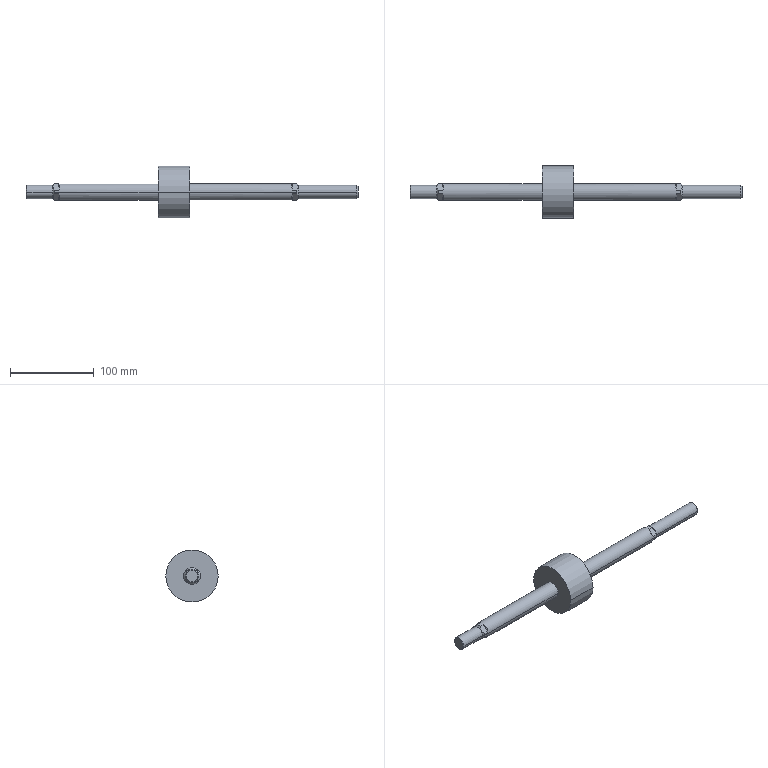Part | SolidWorks | features BaseBody 1 | 1 solid | 38 faces | box 397 x 62.5 x 62.5 mm | volume 216895 mm3 | plane 20 | cylinder 10 | cone 8 | commonest cylinder face diameters 16 x4 20 x4 62.5 x2
STEP:
#1=CARTESIAN_POINT('',(338.773,-8.,0.));
#2=VERTEX_POINT('',#1);
#3=CARTESIAN_POINT('',(338.773,8.,0.));
#4=VERTEX_POINT('',#3);
#5=CARTESIAN_POINT('',(338.773,0.,0.));
#6=DIRECTION('',(-1.,0.,0.));
#7=DIRECTION('',(0.,-1.,0.));
#8=AXIS2_PLACEMENT_3D('',#5,#6,#7);
#9=CIRCLE('',#8,8.);
#10=EDGE_CURVE('',#2,#4,#9,.T.);
#11=ORIENTED_EDGE('',*,*,#10,.T.);
#12=CARTESIAN_POINT('',(269.,8.,0.));
#13=VERTEX_POINT('',#12);
#14=CARTESIAN_POINT('',(340.,8.,0.));
#15=DIRECTION('',(-1.,0.,0.));
#16=VECTOR('',#15,1000.);
#17=LINE('',#14,#16);
#18=EDGE_CURVE('',#4,#13,#17,.T.);
#19=ORIENTED_EDGE('',*,*,#18,.T.);
#20=CARTESIAN_POINT('',(269.,-8.,0.));
#21=VERTEX_POINT('',#20);
#22=CARTESIAN_POINT('',(269.,0.,0.));
#23=DIRECTION('',(-1.,0.,0.));
#24=DIRECTION('',(0.,-1.,0.));
#25=AXIS2_PLACEMENT_3D('',#22,#23,#24);
#26=CIRCLE('',#25,8.);
#27=EDGE_CURVE('',#21,#13,#26,.T.);
#28=ORIENTED_EDGE('',*,*,#27,.F.);
#29=CARTESIAN_POINT('',(340.,-8.,0.));
#30=DIRECTION('',(-1.,0.,0.));
#31=VECTOR('',#30,1000.);
#32=LINE('',#29,#31);
#33=EDGE_CURVE('',#2,#21,#32,.T.);
#34=ORIENTED_EDGE('',*,*,#33,.F.);
#35=EDGE_LOOP('',(#11,#19,#28,#34));
#36=FACE_OUTER_BOUND('',#35,.T.);
#37=CARTESIAN_POINT('',(340.,0.,0.));
#38=DIRECTION('',(-1.,0.,0.));
#39=DIRECTION('',(0.,-1.,0.));
#40=AXIS2_PLACEMENT_3D('',#37,#38,#39);
#41=CYLINDRICAL_SURFACE('',#40,8.);
#42=ADVANCED_FACE('',(#36),#41,.T.);
#43=CARTESIAN_POINT('',(340.,-6.773,0.));
#44=VERTEX_POINT('',#43);
#45=CARTESIAN_POINT('',(340.,6.773,0.));
#46=VERTEX_POINT('',#45);
#47=CARTESIAN_POINT('',(340.,0.,0.));
#48=DIRECTION('',(-1.,0.,0.));
#49=DIRECTION('',(0.,-1.,0.));
#50=AXIS2_PLACEMENT_3D('',#47,#48,#49);
#51=CIRCLE('',#50,6.773);
#52=EDGE_CURVE('',#44,#46,#51,.T.);
#53=ORIENTED_EDGE('',*,*,#52,.T.);
#54=CARTESIAN_POINT('',(340.,6.773,0.));
#55=DIRECTION('',(-0.7071,0.7071,0.));
#56=VECTOR('',#55,1000.);
#57=LINE('',#54,#56);
#58=EDGE_CURVE('',#46,#4,#57,.T.);
#59=ORIENTED_EDGE('',*,*,#58,.T.);
#60=ORIENTED_EDGE('',*,*,#10,.F.);
#61=CARTESIAN_POINT('',(340.,-6.773,0.));
#62=DIRECTION('',(-0.7071,-0.7071,0.));
#63=VECTOR('',#62,1000.);
#64=LINE('',#61,#63);
#65=EDGE_CURVE('',#44,#2,#64,.T.);
#66=ORIENTED_EDGE('',*,*,#65,.F.);
#67=EDGE_LOOP('',(#53,#59,#60,#66));
#68=FACE_OUTER_BOUND('',#67,.T.);
#69=CARTESIAN_POINT('',(340.,0.,0.));
#70=DIRECTION('',(-1.,0.,0.));
#71=DIRECTION('',(0.,-1.,0.));
#72=AXIS2_PLACEMENT_3D('',#69,#70,#71);
#73=CONICAL_SURFACE('',#72,6.773,0.7854);
#74=ADVANCED_FACE('',(#68),#73,.T.);
#75=CARTESIAN_POINT('',(267.,9.735,2.285));
#76=VERTEX_POINT('',#75);
#77=CARTESIAN_POINT('',(267.,10.,0.));
#78=VERTEX_POINT('',#77);
#79=CARTESIAN_POINT('',(267.,0.,0.));
#80=DIRECTION('',(-1.,0.,0.));
#81=DIRECTION('',(0.,-1.,0.));
#82=AXIS2_PLACEMENT_3D('',#79,#80,#81);
#83=CIRCLE('',#82,10.);
#84=EDGE_CURVE('',#76,#78,#83,.T.);
#85=ORIENTED_EDGE('',*,*,#84,.T.);
#86=CARTESIAN_POINT('',(139.,10.,0.));
#87=VERTEX_POINT('',#86);
#88=CARTESIAN_POINT('',(340.,10.,0.));
#89=DIRECTION('',(-1.,0.,0.));
#90=VECTOR('',#89,1000.);
#91=LINE('',#88,#90);
#92=EDGE_CURVE('',#78,#87,#91,.T.);
#93=ORIENTED_EDGE('',*,*,#92,.T.);
#94=CARTESIAN_POINT('',(139.,-10.,0.));
#95=VERTEX_POINT('',#94);
#96=CARTESIAN_POINT('',(139.,0.,0.));
#97=DIRECTION('',(1.,0.,0.));
#98=DIRECTION('',(0.,-1.,0.));
#99=AXIS2_PLACEMENT_3D('',#96,#97,#98);
#100=CIRCLE('',#99,10.);
#101=EDGE_CURVE('',#87,#95,#100,.T.);
#102=ORIENTED_EDGE('',*,*,#101,.T.);
#103=CARTESIAN_POINT('',(267.,-10.,0.));
#104=VERTEX_POINT('',#103);
#105=CARTESIAN_POINT('',(340.,-10.,0.));
#106=DIRECTION('',(-1.,0.,0.));
#107=VECTOR('',#106,1000.);
#108=LINE('',#105,#107);
#109=EDGE_CURVE('',#104,#95,#108,.T.);
#110=ORIENTED_EDGE('',*,*,#109,.F.);
#111=CARTESIAN_POINT('',(267.,-9.735,2.285));
#112=VERTEX_POINT('',#111);
#113=CARTESIAN_POINT('',(267.,0.,0.));
#114=DIRECTION('',(-1.,0.,0.));
#115=DIRECTION('',(0.,-1.,0.));
#116=AXIS2_PLACEMENT_3D('',#113,#114,#115);
#117=CIRCLE('',#116,10.);
#118=EDGE_CURVE('',#104,#112,#117,.T.);
#119=ORIENTED_EDGE('',*,*,#118,.T.);
#120=CARTESIAN_POINT('',(262.,-9.735,2.285));
#121=VERTEX_POINT('',#120);
#122=CARTESIAN_POINT('',(340.,-9.735,2.285));
#123=DIRECTION('',(-1.,0.,0.));
#124=VECTOR('',#123,1000.);
#125=LINE('',#122,#124);
#126=EDGE_CURVE('',#112,#121,#125,.T.);
#127=ORIENTED_EDGE('',*,*,#126,.T.);
#128=CARTESIAN_POINT('',(262.,-2.285,9.735));
#129=VERTEX_POINT('',#128);
#130=CARTESIAN_POINT('',(262.,-9.735,2.285));
#131=CARTESIAN_POINT('',(259.944,-8.844,6.084));
#132=CARTESIAN_POINT('',(259.944,-6.084,8.844));
#133=CARTESIAN_POINT('',(262.,-2.285,9.735));
#134=(BOUNDED_CURVE()B_SPLINE_CURVE(3,(#130,#131,#132,#133),.UNSPECIFIED.,.F.,.F.)B_SPLINE_CURVE_WITH_KNOTS((4,4),(5.728,6.838),.UNSPECIFIED.)CURVE()GEOMETRIC_REPRESENTATION_ITEM()RATIONAL_B_SPLINE_CURVE((1.,0.9,0.9,1.))REPRESENTATION_ITEM(''));
#135=EDGE_CURVE('',#121,#129,#134,.T.);
#136=ORIENTED_EDGE('',*,*,#135,.T.);
#137=CARTESIAN_POINT('',(267.,-2.285,9.735));
#138=VERTEX_POINT('',#137);
#139=CARTESIAN_POINT('',(340.,-2.285,9.735));
#140=DIRECTION('',(1.,0.,0.));
#141=VECTOR('',#140,1000.);
#142=LINE('',#139,#141);
#143=EDGE_CURVE('',#129,#138,#142,.T.);
#144=ORIENTED_EDGE('',*,*,#143,.T.);
#145=CARTESIAN_POINT('',(267.,2.285,9.735));
#146=VERTEX_POINT('',#145);
#147=CARTESIAN_POINT('',(267.,0.,0.));
#148=DIRECTION('',(-1.,0.,0.));
#149=DIRECTION('',(0.,-1.,0.));
#150=AXIS2_PLACEMENT_3D('',#147,#148,#149);
#151=CIRCLE('',#150,10.);
#152=EDGE_CURVE('',#138,#146,#151,.T.);
#153=ORIENTED_EDGE('',*,*,#152,.T.);
#154=CARTESIAN_POINT('',(262.,2.285,9.735));
#155=VERTEX_POINT('',#154);
#156=CARTESIAN_POINT('',(340.,2.285,9.735));
#157=DIRECTION('',(-1.,0.,0.));
#158=VECTOR('',#157,1000.);
#159=LINE('',#156,#158);
#160=EDGE_CURVE('',#146,#155,#159,.T.);
#161=ORIENTED_EDGE('',*,*,#160,.T.);
#162=CARTESIAN_POINT('',(262.,9.735,2.285));
#163=VERTEX_POINT('',#162);
#164=CARTESIAN_POINT('',(262.,2.285,9.735));
#165=CARTESIAN_POINT('',(259.944,6.084,8.844));
#166=CARTESIAN_POINT('',(259.944,8.844,6.084));
#167=CARTESIAN_POINT('',(262.,9.735,2.285));
#168=(BOUNDED_CURVE()B_SPLINE_CURVE(3,(#164,#165,#166,#167),.UNSPECIFIED.,.F.,.F.)B_SPLINE_CURVE_WITH_KNOTS((4,4),(5.728,6.838),.UNSPECIFIED.)CURVE()GEOMETRIC_REPRESENTATION_ITEM()RATIONAL_B_SPLINE_CURVE((1.,0.9,0.9,1.))REPRESENTATION_ITEM(''));
#169=EDGE_CURVE('',#155,#163,#168,.T.);
#170=ORIENTED_EDGE('',*,*,#169,.T.);
#171=CARTESIAN_POINT('',(340.,9.735,2.285));
#172=DIRECTION('',(1.,0.,0.));
#173=VECTOR('',#172,1000.);
#174=LINE('',#171,#173);
#175=EDGE_CURVE('',#163,#76,#174,.T.);
#176=ORIENTED_EDGE('',*,*,#175,.T.);
#177=EDGE_LOOP('',(#85,#93,#102,#110,#119,#127,#136,#144,#153,#161,#170,#176));
#178=FACE_OUTER_BOUND('',#177,.T.);
#179=CARTESIAN_POINT('',(340.,0.,0.));
#180=DIRECTION('',(-1.,0.,0.));
#181=DIRECTION('',(0.,-1.,0.));
#182=AXIS2_PLACEMENT_3D('',#179,#180,#181);
#183=CYLINDRICAL_SURFACE('',#182,10.);
#184=ADVANCED_FACE('',(#178),#183,.T.);
#185=ORIENTED_EDGE('',*,*,#27,.T.);
#186=CARTESIAN_POINT('',(269.,8.,0.));
#187=DIRECTION('',(-0.7071,0.7071,0.));
#188=VECTOR('',#187,1000.);
#189=LINE('',#186,#188);
#190=EDGE_CURVE('',#13,#78,#189,.T.);
#191=ORIENTED_EDGE('',*,*,#190,.T.);
#192=ORIENTED_EDGE('',*,*,#84,.F.);
#193=CARTESIAN_POINT('',(267.,9.735,2.285));
#194=CARTESIAN_POINT('',(267.432,9.156,2.865));
#195=CARTESIAN_POINT('',(267.804,8.561,3.46));
#196=CARTESIAN_POINT('',(268.207,7.629,4.392));
#197=CARTESIAN_POINT('',(268.315,7.31,4.711));
#198=CARTESIAN_POINT('',(268.462,6.66,5.361));
#199=CARTESIAN_POINT('',(268.5,6.336,5.685));
#200=CARTESIAN_POINT('',(268.5,5.686,6.335));
#201=CARTESIAN_POINT('',(268.463,5.362,6.659));
#202=CARTESIAN_POINT('',(268.316,4.713,7.308));
#203=CARTESIAN_POINT('',(268.208,4.393,7.628));
#204=CARTESIAN_POINT('',(267.805,3.46,8.561));
#205=CARTESIAN_POINT('',(267.432,2.865,9.156));
#206=CARTESIAN_POINT('',(267.,2.285,9.735));
#207=B_SPLINE_CURVE_WITH_KNOTS('',3,(#193,#194,#195,#196,#197,#198,#199,#200,#201,#202,#203,#204,#205,#206),.UNSPECIFIED.,.F.,.F.,(4,2,2,2,2,2,4),(0.,0.002753,0.00413,0.005507,0.006884,0.00826,0.01101),.UNSPECIFIED.);
#208=EDGE_CURVE('',#76,#146,#207,.T.);
#209=ORIENTED_EDGE('',*,*,#208,.T.);
#210=ORIENTED_EDGE('',*,*,#152,.F.);
#211=CARTESIAN_POINT('',(267.,-2.285,9.735));
#212=CARTESIAN_POINT('',(267.432,-2.865,9.156));
#213=CARTESIAN_POINT('',(267.804,-3.46,8.561));
#214=CARTESIAN_POINT('',(268.207,-4.392,7.629));
#215=CARTESIAN_POINT('',(268.315,-4.711,7.31));
#216=CARTESIAN_POINT('',(268.462,-5.361,6.66));
#217=CARTESIAN_POINT('',(268.5,-5.685,6.336));
#218=CARTESIAN_POINT('',(268.5,-6.335,5.686));
#219=CARTESIAN_POINT('',(268.463,-6.659,5.362));
#220=CARTESIAN_POINT('',(268.316,-7.308,4.713));
#221=CARTESIAN_POINT('',(268.208,-7.628,4.393));
#222=CARTESIAN_POINT('',(267.805,-8.561,3.46));
#223=CARTESIAN_POINT('',(267.432,-9.156,2.865));
#224=CARTESIAN_POINT('',(267.,-9.735,2.285));
#225=B_SPLINE_CURVE_WITH_KNOTS('',3,(#211,#212,#213,#214,#215,#216,#217,#218,#219,#220,#221,#222,#223,#224),.UNSPECIFIED.,.F.,.F.,(4,2,2,2,2,2,4),(0.,0.002753,0.00413,0.005507,0.006884,0.00826,0.01101),.UNSPECIFIED.);
#226=EDGE_CURVE('',#138,#112,#225,.T.);
#227=ORIENTED_EDGE('',*,*,#226,.T.);
#228=ORIENTED_EDGE('',*,*,#118,.F.);
#229=CARTESIAN_POINT('',(269.,-8.,0.));
#230=DIRECTION('',(-0.7071,-0.7071,0.));
#231=VECTOR('',#230,1000.);
#232=LINE('',#229,#231);
#233=EDGE_CURVE('',#21,#104,#232,.T.);
#234=ORIENTED_EDGE('',*,*,#233,.F.);
#235=EDGE_LOOP('',(#185,#191,#192,#209,#210,#227,#228,#234));
#236=FACE_OUTER_BOUND('',#235,.T.);
#237=CARTESIAN_POINT('',(269.,0.,0.));
#238=DIRECTION('',(-1.,0.,0.));
#239=DIRECTION('',(0.,-1.,0.));
#240=AXIS2_PLACEMENT_3D('',#237,#238,#239);
#241=CONICAL_SURFACE('',#240,8.,0.7854);
#242=ADVANCED_FACE('',(#236),#241,.T.);
#243=CARTESIAN_POINT('',(139.,-31.25,0.));
#244=VERTEX_POINT('',#243);
#245=CARTESIAN_POINT('',(139.,31.25,0.));
#246=VERTEX_POINT('',#245);
#247=CARTESIAN_POINT('',(139.,0.,0.));
#248=DIRECTION('',(-1.,0.,0.));
#249=DIRECTION('',(0.,-1.,0.));
#250=AXIS2_PLACEMENT_3D('',#247,#248,#249);
#251=CIRCLE('',#250,31.25);
#252=EDGE_CURVE('',#244,#246,#251,.T.);
#253=ORIENTED_EDGE('',*,*,#252,.T.);
#254=CARTESIAN_POINT('',(101.,31.25,0.));
#255=VERTEX_POINT('',#254);
#256=CARTESIAN_POINT('',(139.,31.25,0.));
#257=DIRECTION('',(-1.,0.,0.));
#258=VECTOR('',#257,1000.);
#259=LINE('',#256,#258);
#260=EDGE_CURVE('',#246,#255,#259,.T.);
#261=ORIENTED_EDGE('',*,*,#260,.T.);
#262=CARTESIAN_POINT('',(101.,-31.25,0.));
#263=VERTEX_POINT('',#262);
#264=CARTESIAN_POINT('',(101.,0.,0.));
#265=DIRECTION('',(-1.,0.,0.));
#266=DIRECTION('',(0.,-1.,0.));
#267=AXIS2_PLACEMENT_3D('',#264,#265,#266);
#268=CIRCLE('',#267,31.25);
#269=EDGE_CURVE('',#263,#255,#268,.T.);
#270=ORIENTED_EDGE('',*,*,#269,.F.);
#271=CARTESIAN_POINT('',(139.,-31.25,0.));
#272=DIRECTION('',(-1.,0.,0.));
#273=VECTOR('',#272,1000.);
#274=LINE('',#271,#273);
#275=EDGE_CURVE('',#244,#263,#274,.T.);
#276=ORIENTED_EDGE('',*,*,#275,.F.);
#277=EDGE_LOOP('',(#253,#261,#270,#276));
#278=FACE_OUTER_BOUND('',#277,.T.);
#279=CARTESIAN_POINT('',(139.,0.,0.));
#280=DIRECTION('',(-1.,0.,0.));
#281=DIRECTION('',(0.,-1.,0.));
#282=AXIS2_PLACEMENT_3D('',#279,#280,#281);
#283=CYLINDRICAL_SURFACE('',#282,31.25);
#284=ADVANCED_FACE('',(#278),#283,.T.);
#285=CARTESIAN_POINT('',(101.,-10.,0.));
#286=VERTEX_POINT('',#285);
#287=CARTESIAN_POINT('',(101.,10.,0.));
#288=VERTEX_POINT('',#287);
#289=CARTESIAN_POINT('',(101.,0.,0.));
#290=DIRECTION('',(-1.,0.,0.));
#291=DIRECTION('',(0.,-1.,0.));
#292=AXIS2_PLACEMENT_3D('',#289,#290,#291);
#293=CIRCLE('',#292,10.);
#294=EDGE_CURVE('',#286,#288,#293,.T.);
#295=ORIENTED_EDGE('',*,*,#294,.T.);
#296=CARTESIAN_POINT('',(-23.,10.,0.));
#297=VERTEX_POINT('',#296);
#298=CARTESIAN_POINT('',(139.,10.,0.));
#299=DIRECTION('',(-1.,0.,0.));
#300=VECTOR('',#299,1000.);
#301=LINE('',#298,#300);
#302=EDGE_CURVE('',#288,#297,#301,.T.);
#303=ORIENTED_EDGE('',*,*,#302,.T.);
#304=CARTESIAN_POINT('',(-23.,9.735,2.285));
#305=VERTEX_POINT('',#304);
#306=CARTESIAN_POINT('',(-23.,0.,0.));
#307=DIRECTION('',(-1.,0.,0.));
#308=DIRECTION('',(0.,-1.,0.));
#309=AXIS2_PLACEMENT_3D('',#306,#307,#308);
#310=CIRCLE('',#309,10.);
#311=EDGE_CURVE('',#305,#297,#310,.T.);
#312=ORIENTED_EDGE('',*,*,#311,.F.);
#313=CARTESIAN_POINT('',(-18.,9.735,2.285));
#314=VERTEX_POINT('',#313);
#315=CARTESIAN_POINT('',(139.,9.735,2.285));
#316=DIRECTION('',(1.,0.,0.));
#317=VECTOR('',#316,1000.);
#318=LINE('',#315,#317);
#319=EDGE_CURVE('',#305,#314,#318,.T.);
#320=ORIENTED_EDGE('',*,*,#319,.T.);
#321=CARTESIAN_POINT('',(-18.,2.285,9.735));
#322=VERTEX_POINT('',#321);
#323=CARTESIAN_POINT('',(-18.,9.735,2.285));
#324=CARTESIAN_POINT('',(-15.944,8.844,6.084));
#325=CARTESIAN_POINT('',(-15.944,6.084,8.844));
#326=CARTESIAN_POINT('',(-18.,2.285,9.735));
#327=(BOUNDED_CURVE()B_SPLINE_CURVE(3,(#323,#324,#325,#326),.UNSPECIFIED.,.F.,.F.)B_SPLINE_CURVE_WITH_KNOTS((4,4),(2.587,3.696),.UNSPECIFIED.)CURVE()GEOMETRIC_REPRESENTATION_ITEM()RATIONAL_B_SPLINE_CURVE((1.,0.9,0.9,1.))REPRESENTATION_ITEM(''));
#328=EDGE_CURVE('',#314,#322,#327,.T.);
#329=ORIENTED_EDGE('',*,*,#328,.T.);
#330=CARTESIAN_POINT('',(-23.,2.285,9.735));
#331=VERTEX_POINT('',#330);
#332=CARTESIAN_POINT('',(139.,2.285,9.735));
#333=DIRECTION('',(-1.,0.,0.));
#334=VECTOR('',#333,1000.);
#335=LINE('',#332,#334);
#336=EDGE_CURVE('',#322,#331,#335,.T.);
#337=ORIENTED_EDGE('',*,*,#336,.T.);
#338=CARTESIAN_POINT('',(-23.,-2.285,9.735));
#339=VERTEX_POINT('',#338);
#340=CARTESIAN_POINT('',(-23.,0.,0.));
#341=DIRECTION('',(-1.,0.,0.));
#342=DIRECTION('',(0.,-1.,0.));
#343=AXIS2_PLACEMENT_3D('',#340,#341,#342);
#344=CIRCLE('',#343,10.);
#345=EDGE_CURVE('',#339,#331,#344,.T.);
#346=ORIENTED_EDGE('',*,*,#345,.F.);
#347=CARTESIAN_POINT('',(-18.,-2.285,9.735));
#348=VERTEX_POINT('',#347);
#349=CARTESIAN_POINT('',(139.,-2.285,9.735));
#350=DIRECTION('',(1.,0.,0.));
#351=VECTOR('',#350,1000.);
#352=LINE('',#349,#351);
#353=EDGE_CURVE('',#339,#348,#352,.T.);
#354=ORIENTED_EDGE('',*,*,#353,.T.);
#355=CARTESIAN_POINT('',(-18.,-9.735,2.285));
#356=VERTEX_POINT('',#355);
#357=CARTESIAN_POINT('',(-18.,-2.285,9.735));
#358=CARTESIAN_POINT('',(-15.944,-6.084,8.844));
#359=CARTESIAN_POINT('',(-15.944,-8.844,6.084));
#360=CARTESIAN_POINT('',(-18.,-9.735,2.285));
#361=(BOUNDED_CURVE()B_SPLINE_CURVE(3,(#357,#358,#359,#360),.UNSPECIFIED.,.F.,.T.)B_SPLINE_CURVE_WITH_KNOTS((4,4),(2.587,3.696),.UNSPECIFIED.)CURVE()GEOMETRIC_REPRESENTATION_ITEM()RATIONAL_B_SPLINE_CURVE((1.,0.9,0.9,1.))REPRESENTATION_ITEM(''));
#362=EDGE_CURVE('',#348,#356,#361,.T.);
#363=ORIENTED_EDGE('',*,*,#362,.T.);
#364=CARTESIAN_POINT('',(-23.,-9.735,2.285));
#365=VERTEX_POINT('',#364);
#366=CARTESIAN_POINT('',(139.,-9.735,2.285));
#367=DIRECTION('',(-1.,0.,0.));
#368=VECTOR('',#367,1000.);
#369=LINE('',#366,#368);
#370=EDGE_CURVE('',#356,#365,#369,.T.);
#371=ORIENTED_EDGE('',*,*,#370,.T.);
#372=CARTESIAN_POINT('',(-23.,-10.,0.));
#373=VERTEX_POINT('',#372);
#374=CARTESIAN_POINT('',(-23.,0.,0.));
#375=DIRECTION('',(-1.,0.,0.));
#376=DIRECTION('',(0.,-1.,0.));
#377=AXIS2_PLACEMENT_3D('',#374,#375,#376);
#378=CIRCLE('',#377,10.);
#379=EDGE_CURVE('',#373,#365,#378,.T.);
#380=ORIENTED_EDGE('',*,*,#379,.F.);
#381=CARTESIAN_POINT('',(139.,-10.,0.));
#382=DIRECTION('',(-1.,0.,0.));
#383=VECTOR('',#382,1000.);
#384=LINE('',#381,#383);
#385=EDGE_CURVE('',#286,#373,#384,.T.);
#386=ORIENTED_EDGE('',*,*,#385,.F.);
#387=EDGE_LOOP('',(#295,#303,#312,#320,#329,#337,#346,#354,#363,#371,#380,#386));
#388=FACE_OUTER_BOUND('',#387,.T.);
#389=CARTESIAN_POINT('',(139.,0.,0.));
#390=DIRECTION('',(-1.,0.,0.));
#391=DIRECTION('',(0.,-1.,0.));
#392=AXIS2_PLACEMENT_3D('',#389,#390,#391);
#393=CYLINDRICAL_SURFACE('',#392,10.);
#394=ADVANCED_FACE('',(#388),#393,.T.);
#395=CARTESIAN_POINT('',(-25.,-8.,0.));
#396=VERTEX_POINT('',#395);
#397=CARTESIAN_POINT('',(-25.,8.,0.));
#398=VERTEX_POINT('',#397);
#399=CARTESIAN_POINT('',(-25.,0.,0.));
#400=DIRECTION('',(-1.,0.,0.));
#401=DIRECTION('',(0.,-1.,0.));
#402=AXIS2_PLACEMENT_3D('',#399,#400,#401);
#403=CIRCLE('',#402,8.);
#404=EDGE_CURVE('',#396,#398,#403,.T.);
#405=ORIENTED_EDGE('',*,*,#404,.F.);
#406=CARTESIAN_POINT('',(-23.,-10.,0.));
#407=DIRECTION('',(0.7071,-0.7071,0.));
#408=VECTOR('',#407,1000.);
#409=LINE('',#406,#408);
#410=EDGE_CURVE('',#396,#373,#409,.T.);
#411=ORIENTED_EDGE('',*,*,#410,.T.);
#412=ORIENTED_EDGE('',*,*,#379,.T.);
#413=CARTESIAN_POINT('',(-23.,-9.735,2.285));
#414=CARTESIAN_POINT('',(-23.432,-9.156,2.865));
#415=CARTESIAN_POINT('',(-23.804,-8.561,3.46));
#416=CARTESIAN_POINT('',(-24.207,-7.629,4.392));
#417=CARTESIAN_POINT('',(-24.315,-7.31,4.711));
#418=CARTESIAN_POINT('',(-24.462,-6.66,5.361));
#419=CARTESIAN_POINT('',(-24.5,-6.336,5.685));
#420=CARTESIAN_POINT('',(-24.5,-5.686,6.335));
#421=CARTESIAN_POINT('',(-24.463,-5.362,6.659));
#422=CARTESIAN_POINT('',(-24.316,-4.713,7.308));
#423=CARTESIAN_POINT('',(-24.208,-4.393,7.628));
#424=CARTESIAN_POINT('',(-23.805,-3.46,8.561));
#425=CARTESIAN_POINT('',(-23.432,-2.865,9.156));
#426=CARTESIAN_POINT('',(-23.,-2.285,9.735));
#427=B_SPLINE_CURVE_WITH_KNOTS('',3,(#413,#414,#415,#416,#417,#418,#419,#420,#421,#422,#423,#424,#425,#426),.UNSPECIFIED.,.F.,.F.,(4,2,2,2,2,2,4),(0.,0.002753,0.00413,0.005507,0.006884,0.00826,0.01101),.UNSPECIFIED.);
#428=EDGE_CURVE('',#365,#339,#427,.T.);
#429=ORIENTED_EDGE('',*,*,#428,.T.);
#430=ORIENTED_EDGE('',*,*,#345,.T.);
#431=CARTESIAN_POINT('',(-23.,2.285,9.735));
#432=CARTESIAN_POINT('',(-23.432,2.865,9.156));
#433=CARTESIAN_POINT('',(-23.804,3.46,8.561));
#434=CARTESIAN_POINT('',(-24.207,4.392,7.629));
#435=CARTESIAN_POINT('',(-24.315,4.711,7.31));
#436=CARTESIAN_POINT('',(-24.462,5.361,6.66));
#437=CARTESIAN_POINT('',(-24.5,5.685,6.336));
#438=CARTESIAN_POINT('',(-24.5,6.335,5.686));
#439=CARTESIAN_POINT('',(-24.463,6.659,5.362));
#440=CARTESIAN_POINT('',(-24.316,7.308,4.713));
#441=CARTESIAN_POINT('',(-24.208,7.628,4.393));
#442=CARTESIAN_POINT('',(-23.805,8.561,3.46));
#443=CARTESIAN_POINT('',(-23.432,9.156,2.865));
#444=CARTESIAN_POINT('',(-23.,9.735,2.285));
#445=B_SPLINE_CURVE_WITH_KNOTS('',3,(#431,#432,#433,#434,#435,#436,#437,#438,#439,#440,#441,#442,#443,#444),.UNSPECIFIED.,.F.,.F.,(4,2,2,2,2,2,4),(0.,0.002753,0.00413,0.005507,0.006884,0.00826,0.01101),.UNSPECIFIED.);
#446=EDGE_CURVE('',#331,#305,#445,.T.);
#447=ORIENTED_EDGE('',*,*,#446,.T.);
#448=ORIENTED_EDGE('',*,*,#311,.T.);
#449=CARTESIAN_POINT('',(-23.,10.,0.));
#450=DIRECTION('',(0.7071,0.7071,0.));
#451=VECTOR('',#450,1000.);
#452=LINE('',#449,#451);
#453=EDGE_CURVE('',#398,#297,#452,.T.);
#454=ORIENTED_EDGE('',*,*,#453,.F.);
#455=EDGE_LOOP('',(#405,#411,#412,#429,#430,#447,#448,#454));
#456=FACE_OUTER_BOUND('',#455,.T.);
#457=CARTESIAN_POINT('',(-23.,0.,0.));
#458=DIRECTION('',(1.,0.,0.));
#459=DIRECTION('',(0.,1.,0.));
#460=AXIS2_PLACEMENT_3D('',#457,#458,#459);
#461=CONICAL_SURFACE('',#460,10.,0.7854);
#462=ADVANCED_FACE('',(#456),#461,.T.);
#463=ORIENTED_EDGE('',*,*,#404,.T.);
#464=CARTESIAN_POINT('',(-56.08,8.,0.));
#465=VERTEX_POINT('',#464);
#466=CARTESIAN_POINT('',(139.,8.,0.));
#467=DIRECTION('',(-1.,0.,0.));
#468=VECTOR('',#467,1000.);
#469=LINE('',#466,#468);
#470=EDGE_CURVE('',#398,#465,#469,.T.);
#471=ORIENTED_EDGE('',*,*,#470,.T.);
#472=CARTESIAN_POINT('',(-56.08,-8.,0.));
#473=VERTEX_POINT('',#472);
#474=CARTESIAN_POINT('',(-56.08,0.,0.));
#475=DIRECTION('',(-1.,0.,0.));
#476=DIRECTION('',(0.,-1.,0.));
#477=AXIS2_PLACEMENT_3D('',#474,#475,#476);
#478=CIRCLE('',#477,8.);
#479=EDGE_CURVE('',#473,#465,#478,.T.);
#480=ORIENTED_EDGE('',*,*,#479,.F.);
#481=CARTESIAN_POINT('',(139.,-8.,0.));
#482=DIRECTION('',(-1.,0.,0.));
#483=VECTOR('',#482,1000.);
#484=LINE('',#481,#483);
#485=EDGE_CURVE('',#396,#473,#484,.T.);
#486=ORIENTED_EDGE('',*,*,#485,.F.);
#487=EDGE_LOOP('',(#463,#471,#480,#486));
#488=FACE_OUTER_BOUND('',#487,.T.);
#489=CARTESIAN_POINT('',(139.,0.,0.));
#490=DIRECTION('',(-1.,0.,0.));
#491=DIRECTION('',(0.,-1.,0.));
#492=AXIS2_PLACEMENT_3D('',#489,#490,#491);
#493=CYLINDRICAL_SURFACE('',#492,8.);
#494=ADVANCED_FACE('',(#488),#493,.T.);
#495=CARTESIAN_POINT('',(-57.,-7.08,0.));
#496=VERTEX_POINT('',#495);
#497=CARTESIAN_POINT('',(-57.,7.08,0.));
#498=VERTEX_POINT('',#497);
#499=CARTESIAN_POINT('',(-57.,0.,0.));
#500=DIRECTION('',(-1.,0.,0.));
#501=DIRECTION('',(0.,-1.,0.));
#502=AXIS2_PLACEMENT_3D('',#499,#500,#501);
#503=CIRCLE('',#502,7.08);
#504=EDGE_CURVE('',#496,#498,#503,.T.);
#505=ORIENTED_EDGE('',*,*,#504,.F.);
#506=CARTESIAN_POINT('',(-56.08,-8.,0.));
#507=DIRECTION('',(0.7071,-0.7071,0.));
#508=VECTOR('',#507,1000.);
#509=LINE('',#506,#508);
#510=EDGE_CURVE('',#496,#473,#509,.T.);
#511=ORIENTED_EDGE('',*,*,#510,.T.);
#512=ORIENTED_EDGE('',*,*,#479,.T.);
#513=CARTESIAN_POINT('',(-56.08,8.,0.));
#514=DIRECTION('',(0.7071,0.7071,0.));
#515=VECTOR('',#514,1000.);
#516=LINE('',#513,#515);
#517=EDGE_CURVE('',#498,#465,#516,.T.);
#518=ORIENTED_EDGE('',*,*,#517,.F.);
#519=EDGE_LOOP('',(#505,#511,#512,#518));
#520=FACE_OUTER_BOUND('',#519,.T.);
#521=CARTESIAN_POINT('',(-56.08,0.,0.));
#522=DIRECTION('',(1.,0.,0.));
#523=DIRECTION('',(0.,1.,0.));
#524=AXIS2_PLACEMENT_3D('',#521,#522,#523);
#525=CONICAL_SURFACE('',#524,8.,0.7854);
#526=ADVANCED_FACE('',(#520),#525,.T.);
#527=CARTESIAN_POINT('',(267.,2.285,-9.735));
#528=VERTEX_POINT('',#527);
#529=CARTESIAN_POINT('',(267.,9.735,-2.285));
#530=VERTEX_POINT('',#529);
#531=CARTESIAN_POINT('',(267.,2.285,-9.735));
#532=CARTESIAN_POINT('',(267.432,2.865,-9.156));
#533=CARTESIAN_POINT('',(267.804,3.46,-8.561));
#534=CARTESIAN_POINT('',(268.207,4.392,-7.629));
#535=CARTESIAN_POINT('',(268.315,4.711,-7.31));
#536=CARTESIAN_POINT('',(268.462,5.361,-6.66));
#537=CARTESIAN_POINT('',(268.5,5.685,-6.336));
#538=CARTESIAN_POINT('',(268.5,6.335,-5.686));
#539=CARTESIAN_POINT('',(268.463,6.659,-5.362));
#540=CARTESIAN_POINT('',(268.316,7.308,-4.713));
#541=CARTESIAN_POINT('',(268.208,7.628,-4.393));
#542=CARTESIAN_POINT('',(267.805,8.561,-3.46));
#543=CARTESIAN_POINT('',(267.432,9.156,-2.865));
#544=CARTESIAN_POINT('',(267.,9.735,-2.285));
#545=B_SPLINE_CURVE_WITH_KNOTS('',3,(#531,#532,#533,#534,#535,#536,#537,#538,#539,#540,#541,#542,#543,#544),.UNSPECIFIED.,.F.,.F.,(4,2,2,2,2,2,4),(0.,0.002753,0.00413,0.005507,0.006884,0.00826,0.01101),.UNSPECIFIED.);
#546=EDGE_CURVE('',#528,#530,#545,.T.);
#547=ORIENTED_EDGE('',*,*,#546,.F.);
#548=CARTESIAN_POINT('',(262.,2.285,-9.735));
#549=VERTEX_POINT('',#548);
#550=CARTESIAN_POINT('',(340.,2.285,-9.735));
#551=DIRECTION('',(1.,0.,0.));
#552=VECTOR('',#551,1000.);
#553=LINE('',#550,#552);
#554=EDGE_CURVE('',#549,#528,#553,.T.);
#555=ORIENTED_EDGE('',*,*,#554,.F.);
#556=CARTESIAN_POINT('',(262.,9.735,-2.285));
#557=VERTEX_POINT('',#556);
#558=CARTESIAN_POINT('',(262.,18.031,6.01));
#559=DIRECTION('',(0.,-0.7071,-0.7071));
#560=VECTOR('',#559,1000.);
#561=LINE('',#558,#560);
#562=EDGE_CURVE('',#557,#549,#561,.T.);
#563=ORIENTED_EDGE('',*,*,#562,.F.);
#564=CARTESIAN_POINT('',(340.,9.735,-2.285));
#565=DIRECTION('',(-1.,0.,0.));
#566=VECTOR('',#565,1000.);
#567=LINE('',#564,#566);
#568=EDGE_CURVE('',#530,#557,#567,.T.);
#569=ORIENTED_EDGE('',*,*,#568,.F.);
#570=EDGE_LOOP('',(#547,#555,#563,#569));
#571=FACE_OUTER_BOUND('',#570,.T.);
#572=CARTESIAN_POINT('',(341.,18.031,6.01));
#573=DIRECTION('',(0.,-0.7071,0.7071));
#574=DIRECTION('',(-1.,0.,0.));
#575=AXIS2_PLACEMENT_3D('',#572,#573,#574);
#576=PLANE('',#575);
#577=ADVANCED_FACE('',(#571),#576,.F.);
#578=CARTESIAN_POINT('',(262.,9.735,-2.285));
#579=CARTESIAN_POINT('',(259.944,8.844,-6.084));
#580=CARTESIAN_POINT('',(259.944,6.084,-8.844));
#581=CARTESIAN_POINT('',(262.,2.285,-9.735));
#582=(BOUNDED_CURVE()B_SPLINE_CURVE(3,(#578,#579,#580,#581),.UNSPECIFIED.,.F.,.F.)B_SPLINE_CURVE_WITH_KNOTS((4,4),(5.728,6.838),.UNSPECIFIED.)CURVE()GEOMETRIC_REPRESENTATION_ITEM()RATIONAL_B_SPLINE_CURVE((1.,0.9,0.9,1.))REPRESENTATION_ITEM(''));
#583=EDGE_CURVE('',#557,#549,#582,.T.);
#584=ORIENTED_EDGE('',*,*,#583,.F.);
#585=ORIENTED_EDGE('',*,*,#562,.T.);
#586=EDGE_LOOP('',(#584,#585));
#587=FACE_OUTER_BOUND('',#586,.T.);
#588=CARTESIAN_POINT('',(262.,18.031,6.01));
#589=DIRECTION('',(-0.7071,-0.5,0.5));
#590=DIRECTION('',(-0.5774,0.8165,0.));
#591=AXIS2_PLACEMENT_3D('',#588,#589,#590);
#592=PLANE('',#591);
#593=ADVANCED_FACE('',(#587),#592,.F.);
#594=ORIENTED_EDGE('',*,*,#226,.F.);
#595=ORIENTED_EDGE('',*,*,#143,.F.);
#596=CARTESIAN_POINT('',(262.,6.01,18.031));
#597=DIRECTION('',(0.,-0.7071,-0.7071));
#598=VECTOR('',#597,1000.);
#599=LINE('',#596,#598);
#600=EDGE_CURVE('',#129,#121,#599,.T.);
#601=ORIENTED_EDGE('',*,*,#600,.T.);
#602=ORIENTED_EDGE('',*,*,#126,.F.);
#603=EDGE_LOOP('',(#594,#595,#601,#602));
#604=FACE_OUTER_BOUND('',#603,.T.);
#605=CARTESIAN_POINT('',(262.,6.01,18.031));
#606=DIRECTION('',(0.,0.7071,-0.7071));
#607=DIRECTION('',(-1.,0.,0.));
#608=AXIS2_PLACEMENT_3D('',#605,#606,#607);
#609=PLANE('',#608);
#610=ADVANCED_FACE('',(#604),#609,.F.);
#611=ORIENTED_EDGE('',*,*,#135,.F.);
#612=ORIENTED_EDGE('',*,*,#600,.F.);
#613=EDGE_LOOP('',(#611,#612));
#614=FACE_OUTER_BOUND('',#613,.T.);
#615=CARTESIAN_POINT('',(260.5,4.95,19.092));
#616=DIRECTION('',(-0.7071,0.5,-0.5));
#617=DIRECTION('',(-0.5774,0.,0.8165));
#618=AXIS2_PLACEMENT_3D('',#615,#616,#617);
#619=PLANE('',#618);
#620=ADVANCED_FACE('',(#614),#619,.F.);
#621=CARTESIAN_POINT('',(267.,-9.735,-2.285));
#622=VERTEX_POINT('',#621);
#623=CARTESIAN_POINT('',(267.,-2.285,-9.735));
#624=VERTEX_POINT('',#623);
#625=CARTESIAN_POINT('',(267.,-9.735,-2.285));
#626=CARTESIAN_POINT('',(267.432,-9.156,-2.865));
#627=CARTESIAN_POINT('',(267.804,-8.561,-3.46));
#628=CARTESIAN_POINT('',(268.207,-7.629,-4.392));
#629=CARTESIAN_POINT('',(268.315,-7.31,-4.711));
#630=CARTESIAN_POINT('',(268.462,-6.66,-5.361));
#631=CARTESIAN_POINT('',(268.5,-6.336,-5.685));
#632=CARTESIAN_POINT('',(268.5,-5.686,-6.335));
#633=CARTESIAN_POINT('',(268.463,-5.362,-6.659));
#634=CARTESIAN_POINT('',(268.316,-4.713,-7.308));
#635=CARTESIAN_POINT('',(268.208,-4.393,-7.628));
#636=CARTESIAN_POINT('',(267.805,-3.46,-8.561));
#637=CARTESIAN_POINT('',(267.432,-2.865,-9.156));
#638=CARTESIAN_POINT('',(267.,-2.285,-9.735));
#639=B_SPLINE_CURVE_WITH_KNOTS('',3,(#625,#626,#627,#628,#629,#630,#631,#632,#633,#634,#635,#636,#637,#638),.UNSPECIFIED.,.F.,.F.,(4,2,2,2,2,2,4),(0.,0.002753,0.00413,0.005507,0.006884,0.00826,0.01101),.UNSPECIFIED.);
#640=EDGE_CURVE('',#622,#624,#639,.T.);
#641=ORIENTED_EDGE('',*,*,#640,.F.);
#642=CARTESIAN_POINT('',(262.,-9.735,-2.285));
#643=VERTEX_POINT('',#642);
#644=CARTESIAN_POINT('',(340.,-9.735,-2.285));
#645=DIRECTION('',(1.,0.,0.));
#646=VECTOR('',#645,1000.);
#647=LINE('',#644,#646);
#648=EDGE_CURVE('',#643,#622,#647,.T.);
#649=ORIENTED_EDGE('',*,*,#648,.F.);
#650=CARTESIAN_POINT('',(262.,-2.285,-9.735));
#651=VERTEX_POINT('',#650);
#652=CARTESIAN_POINT('',(262.,6.01,-18.031));
#653=DIRECTION('',(0.,-0.7071,0.7071));
#654=VECTOR('',#653,1000.);
#655=LINE('',#652,#654);
#656=EDGE_CURVE('',#651,#643,#655,.T.);
#657=ORIENTED_EDGE('',*,*,#656,.F.);
#658=CARTESIAN_POINT('',(340.,-2.285,-9.735));
#659=DIRECTION('',(-1.,0.,0.));
#660=VECTOR('',#659,1000.);
#661=LINE('',#658,#660);
#662=EDGE_CURVE('',#624,#651,#661,.T.);
#663=ORIENTED_EDGE('',*,*,#662,.F.);
#664=EDGE_LOOP('',(#641,#649,#657,#663));
#665=FACE_OUTER_BOUND('',#664,.T.);
#666=CARTESIAN_POINT('',(341.,6.01,-18.031));
#667=DIRECTION('',(0.,0.7071,0.7071));
#668=DIRECTION('',(1.,0.,0.));
#669=AXIS2_PLACEMENT_3D('',#666,#667,#668);
#670=PLANE('',#669);
#671=ADVANCED_FACE('',(#665),#670,.F.);
#672=CARTESIAN_POINT('',(262.,-2.285,-9.735));
#673=CARTESIAN_POINT('',(259.944,-6.084,-8.844));
#674=CARTESIAN_POINT('',(259.944,-8.844,-6.084));
#675=CARTESIAN_POINT('',(262.,-9.735,-2.285));
#676=(BOUNDED_CURVE()B_SPLINE_CURVE(3,(#672,#673,#674,#675),.UNSPECIFIED.,.F.,.F.)B_SPLINE_CURVE_WITH_KNOTS((4,4),(5.728,6.838),.UNSPECIFIED.)CURVE()GEOMETRIC_REPRESENTATION_ITEM()RATIONAL_B_SPLINE_CURVE((1.,0.9,0.9,1.))REPRESENTATION_ITEM(''));
#677=EDGE_CURVE('',#651,#643,#676,.T.);
#678=ORIENTED_EDGE('',*,*,#677,.F.);
#679=ORIENTED_EDGE('',*,*,#656,.T.);
#680=EDGE_LOOP('',(#678,#679));
#681=FACE_OUTER_BOUND('',#680,.T.);
#682=CARTESIAN_POINT('',(262.,6.01,-18.031));
#683=DIRECTION('',(-0.7071,0.5,0.5));
#684=DIRECTION('',(0.5774,0.,0.8165));
#685=AXIS2_PLACEMENT_3D('',#682,#683,#684);
#686=PLANE('',#685);
#687=ADVANCED_FACE('',(#681),#686,.F.);
#688=ORIENTED_EDGE('',*,*,#208,.F.);
#689=ORIENTED_EDGE('',*,*,#175,.F.);
#690=CARTESIAN_POINT('',(262.,18.031,-6.01));
#691=DIRECTION('',(0.,-0.7071,0.7071));
#692=VECTOR('',#691,1000.);
#693=LINE('',#690,#692);
#694=EDGE_CURVE('',#163,#155,#693,.T.);
#695=ORIENTED_EDGE('',*,*,#694,.T.);
#696=ORIENTED_EDGE('',*,*,#160,.F.);
#697=EDGE_LOOP('',(#688,#689,#695,#696));
#698=FACE_OUTER_BOUND('',#697,.T.);
#699=CARTESIAN_POINT('',(262.,18.031,-6.01));
#700=DIRECTION('',(0.,-0.7071,-0.7071));
#701=DIRECTION('',(0.,0.7071,-0.7071));
#702=AXIS2_PLACEMENT_3D('',#699,#700,#701);
#703=PLANE('',#702);
#704=ADVANCED_FACE('',(#698),#703,.F.);
#705=ORIENTED_EDGE('',*,*,#169,.F.);
#706=ORIENTED_EDGE('',*,*,#694,.F.);
#707=EDGE_LOOP('',(#705,#706));
#708=FACE_OUTER_BOUND('',#707,.T.);
#709=CARTESIAN_POINT('',(260.5,19.092,-4.95));
#710=DIRECTION('',(-0.7071,-0.5,-0.5));
#711=DIRECTION('',(-0.5774,0.,0.8165));
#712=AXIS2_PLACEMENT_3D('',#709,#710,#711);
#713=PLANE('',#712);
#714=ADVANCED_FACE('',(#708),#713,.F.);
#715=ORIENTED_EDGE('',*,*,#52,.F.);
#716=CARTESIAN_POINT('',(340.,0.,0.));
#717=DIRECTION('',(-1.,0.,0.));
#718=DIRECTION('',(0.,-1.,0.));
#719=AXIS2_PLACEMENT_3D('',#716,#717,#718);
#720=CIRCLE('',#719,6.773);
#721=EDGE_CURVE('',#46,#44,#720,.T.);
#722=ORIENTED_EDGE('',*,*,#721,.F.);
#723=EDGE_LOOP('',(#715,#722));
#724=FACE_OUTER_BOUND('',#723,.T.);
#725=CARTESIAN_POINT('',(340.,6.773,0.));
#726=DIRECTION('',(-1.,0.,0.));
#727=DIRECTION('',(0.,1.,0.));
#728=AXIS2_PLACEMENT_3D('',#725,#726,#727);
#729=PLANE('',#728);
#730=ADVANCED_FACE('',(#724),#729,.F.);
#731=CARTESIAN_POINT('',(-18.,6.01,18.031));
#732=DIRECTION('',(0.,-0.7071,-0.7071));
#733=VECTOR('',#732,1000.);
#734=LINE('',#731,#733);
#735=EDGE_CURVE('',#348,#356,#734,.T.);
#736=ORIENTED_EDGE('',*,*,#735,.F.);
#737=ORIENTED_EDGE('',*,*,#353,.F.);
#738=ORIENTED_EDGE('',*,*,#428,.F.);
#739=ORIENTED_EDGE('',*,*,#370,.F.);
#740=EDGE_LOOP('',(#736,#737,#738,#739));
#741=FACE_OUTER_BOUND('',#740,.T.);
#742=CARTESIAN_POINT('',(-57.,6.01,18.031));
#743=DIRECTION('',(0.,0.7071,-0.7071));
#744=DIRECTION('',(-1.,0.,0.));
#745=AXIS2_PLACEMENT_3D('',#742,#743,#744);
#746=PLANE('',#745);
#747=ADVANCED_FACE('',(#741),#746,.F.);
#748=ORIENTED_EDGE('',*,*,#735,.T.);
#749=ORIENTED_EDGE('',*,*,#362,.F.);
#750=EDGE_LOOP('',(#748,#749));
#751=FACE_OUTER_BOUND('',#750,.T.);
#752=CARTESIAN_POINT('',(-18.,6.01,18.031));
#753=DIRECTION('',(0.7071,0.5,-0.5));
#754=DIRECTION('',(0.,-0.7071,-0.7071));
#755=AXIS2_PLACEMENT_3D('',#752,#753,#754);
#756=PLANE('',#755);
#757=ADVANCED_FACE('',(#751),#756,.F.);
#758=CARTESIAN_POINT('',(-18.,9.735,-2.285));
#759=VERTEX_POINT('',#758);
#760=CARTESIAN_POINT('',(-18.,2.285,-9.735));
#761=VERTEX_POINT('',#760);
#762=CARTESIAN_POINT('',(-18.,18.031,6.01));
#763=DIRECTION('',(0.,-0.7071,-0.7071));
#764=VECTOR('',#763,1000.);
#765=LINE('',#762,#764);
#766=EDGE_CURVE('',#759,#761,#765,.T.);
#767=ORIENTED_EDGE('',*,*,#766,.T.);
#768=CARTESIAN_POINT('',(-23.,2.285,-9.735));
#769=VERTEX_POINT('',#768);
#770=CARTESIAN_POINT('',(139.,2.285,-9.735));
#771=DIRECTION('',(1.,0.,0.));
#772=VECTOR('',#771,1000.);
#773=LINE('',#770,#772);
#774=EDGE_CURVE('',#769,#761,#773,.T.);
#775=ORIENTED_EDGE('',*,*,#774,.F.);
#776=CARTESIAN_POINT('',(-23.,9.735,-2.285));
#777=VERTEX_POINT('',#776);
#778=CARTESIAN_POINT('',(-23.,9.735,-2.285));
#779=CARTESIAN_POINT('',(-23.432,9.156,-2.865));
#780=CARTESIAN_POINT('',(-23.804,8.561,-3.46));
#781=CARTESIAN_POINT('',(-24.207,7.629,-4.392));
#782=CARTESIAN_POINT('',(-24.315,7.31,-4.711));
#783=CARTESIAN_POINT('',(-24.462,6.66,-5.361));
#784=CARTESIAN_POINT('',(-24.5,6.336,-5.685));
#785=CARTESIAN_POINT('',(-24.5,5.686,-6.335));
#786=CARTESIAN_POINT('',(-24.463,5.362,-6.659));
#787=CARTESIAN_POINT('',(-24.316,4.713,-7.308));
#788=CARTESIAN_POINT('',(-24.208,4.393,-7.628));
#789=CARTESIAN_POINT('',(-23.805,3.46,-8.561));
#790=CARTESIAN_POINT('',(-23.432,2.865,-9.156));
#791=CARTESIAN_POINT('',(-23.,2.285,-9.735));
#792=B_SPLINE_CURVE_WITH_KNOTS('',3,(#778,#779,#780,#781,#782,#783,#784,#785,#786,#787,#788,#789,#790,#791),.UNSPECIFIED.,.F.,.F.,(4,2,2,2,2,2,4),(0.,0.002753,0.00413,0.005507,0.006884,0.00826,0.01101),.UNSPECIFIED.);
#793=EDGE_CURVE('',#777,#769,#792,.T.);
#794=ORIENTED_EDGE('',*,*,#793,.F.);
#795=CARTESIAN_POINT('',(139.,9.735,-2.285));
#796=DIRECTION('',(-1.,0.,0.));
#797=VECTOR('',#796,1000.);
#798=LINE('',#795,#797);
#799=EDGE_CURVE('',#759,#777,#798,.T.);
#800=ORIENTED_EDGE('',*,*,#799,.F.);
#801=EDGE_LOOP('',(#767,#775,#794,#800));
#802=FACE_OUTER_BOUND('',#801,.T.);
#803=CARTESIAN_POINT('',(-18.,18.031,6.01));
#804=DIRECTION('',(0.,-0.7071,0.7071));
#805=DIRECTION('',(-1.,0.,0.));
#806=AXIS2_PLACEMENT_3D('',#803,#804,#805);
#807=PLANE('',#806);
#808=ADVANCED_FACE('',(#802),#807,.F.);
#809=ORIENTED_EDGE('',*,*,#766,.F.);
#810=CARTESIAN_POINT('',(-18.,2.285,-9.735));
#811=CARTESIAN_POINT('',(-15.944,6.084,-8.844));
#812=CARTESIAN_POINT('',(-15.944,8.844,-6.084));
#813=CARTESIAN_POINT('',(-18.,9.735,-2.285));
#814=(BOUNDED_CURVE()B_SPLINE_CURVE(3,(#810,#811,#812,#813),.UNSPECIFIED.,.F.,.T.)B_SPLINE_CURVE_WITH_KNOTS((4,4),(2.587,3.696),.UNSPECIFIED.)CURVE()GEOMETRIC_REPRESENTATION_ITEM()RATIONAL_B_SPLINE_CURVE((1.,0.9,0.9,1.))REPRESENTATION_ITEM(''));
#815=EDGE_CURVE('',#761,#759,#814,.T.);
#816=ORIENTED_EDGE('',*,*,#815,.F.);
#817=EDGE_LOOP('',(#809,#816));
#818=FACE_OUTER_BOUND('',#817,.T.);
#819=CARTESIAN_POINT('',(-1.,30.052,-6.01));
#820=DIRECTION('',(0.7071,-0.5,0.5));
#821=DIRECTION('',(0.,-0.7071,-0.7071));
#822=AXIS2_PLACEMENT_3D('',#819,#820,#821);
#823=PLANE('',#822);
#824=ADVANCED_FACE('',(#818),#823,.F.);
#825=CARTESIAN_POINT('',(-18.,18.031,-6.01));
#826=DIRECTION('',(0.,-0.7071,0.7071));
#827=VECTOR('',#826,1000.);
#828=LINE('',#825,#827);
#829=EDGE_CURVE('',#314,#322,#828,.T.);
#830=ORIENTED_EDGE('',*,*,#829,.F.);
#831=ORIENTED_EDGE('',*,*,#319,.F.);
#832=ORIENTED_EDGE('',*,*,#446,.F.);
#833=ORIENTED_EDGE('',*,*,#336,.F.);
#834=EDGE_LOOP('',(#830,#831,#832,#833));
#835=FACE_OUTER_BOUND('',#834,.T.);
#836=CARTESIAN_POINT('',(-57.,18.031,-6.01));
#837=DIRECTION('',(0.,-0.7071,-0.7071));
#838=DIRECTION('',(0.,0.7071,-0.7071));
#839=AXIS2_PLACEMENT_3D('',#836,#837,#838);
#840=PLANE('',#839);
#841=ADVANCED_FACE('',(#835),#840,.F.);
#842=ORIENTED_EDGE('',*,*,#829,.T.);
#843=ORIENTED_EDGE('',*,*,#328,.F.);
#844=EDGE_LOOP('',(#842,#843));
#845=FACE_OUTER_BOUND('',#844,.T.);
#846=CARTESIAN_POINT('',(-18.,18.031,-6.01));
#847=DIRECTION('',(0.7071,-0.5,-0.5));
#848=DIRECTION('',(0.,-0.7071,0.7071));
#849=AXIS2_PLACEMENT_3D('',#846,#847,#848);
#850=PLANE('',#849);
#851=ADVANCED_FACE('',(#845),#850,.F.);
#852=CARTESIAN_POINT('',(-18.,-2.285,-9.735));
#853=VERTEX_POINT('',#852);
#854=CARTESIAN_POINT('',(-18.,-9.735,-2.285));
#855=VERTEX_POINT('',#854);
#856=CARTESIAN_POINT('',(-18.,6.01,-18.031));
#857=DIRECTION('',(0.,-0.7071,0.7071));
#858=VECTOR('',#857,1000.);
#859=LINE('',#856,#858);
#860=EDGE_CURVE('',#853,#855,#859,.T.);
#861=ORIENTED_EDGE('',*,*,#860,.T.);
#862=CARTESIAN_POINT('',(-23.,-9.735,-2.285));
#863=VERTEX_POINT('',#862);
#864=CARTESIAN_POINT('',(139.,-9.735,-2.285));
#865=DIRECTION('',(1.,0.,0.));
#866=VECTOR('',#865,1000.);
#867=LINE('',#864,#866);
#868=EDGE_CURVE('',#863,#855,#867,.T.);
#869=ORIENTED_EDGE('',*,*,#868,.F.);
#870=CARTESIAN_POINT('',(-23.,-2.285,-9.735));
#871=VERTEX_POINT('',#870);
#872=CARTESIAN_POINT('',(-23.,-2.285,-9.735));
#873=CARTESIAN_POINT('',(-23.432,-2.865,-9.156));
#874=CARTESIAN_POINT('',(-23.804,-3.46,-8.561));
#875=CARTESIAN_POINT('',(-24.207,-4.392,-7.629));
#876=CARTESIAN_POINT('',(-24.315,-4.711,-7.31));
#877=CARTESIAN_POINT('',(-24.462,-5.361,-6.66));
#878=CARTESIAN_POINT('',(-24.5,-5.685,-6.336));
#879=CARTESIAN_POINT('',(-24.5,-6.335,-5.686));
#880=CARTESIAN_POINT('',(-24.463,-6.659,-5.362));
#881=CARTESIAN_POINT('',(-24.316,-7.308,-4.713));
#882=CARTESIAN_POINT('',(-24.208,-7.628,-4.393));
#883=CARTESIAN_POINT('',(-23.805,-8.561,-3.46));
#884=CARTESIAN_POINT('',(-23.432,-9.156,-2.865));
#885=CARTESIAN_POINT('',(-23.,-9.735,-2.285));
#886=B_SPLINE_CURVE_WITH_KNOTS('',3,(#872,#873,#874,#875,#876,#877,#878,#879,#880,#881,#882,#883,#884,#885),.UNSPECIFIED.,.F.,.F.,(4,2,2,2,2,2,4),(0.,0.002753,0.00413,0.005507,0.006884,0.00826,0.01101),.UNSPECIFIED.);
#887=EDGE_CURVE('',#871,#863,#886,.T.);
#888=ORIENTED_EDGE('',*,*,#887,.F.);
#889=CARTESIAN_POINT('',(139.,-2.285,-9.735));
#890=DIRECTION('',(-1.,0.,0.));
#891=VECTOR('',#890,1000.);
#892=LINE('',#889,#891);
#893=EDGE_CURVE('',#853,#871,#892,.T.);
#894=ORIENTED_EDGE('',*,*,#893,.F.);
#895=EDGE_LOOP('',(#861,#869,#888,#894));
#896=FACE_OUTER_BOUND('',#895,.T.);
#897=CARTESIAN_POINT('',(-18.,6.01,-18.031));
#898=DIRECTION('',(0.,0.7071,0.7071));
#899=DIRECTION('',(1.,0.,0.));
#900=AXIS2_PLACEMENT_3D('',#897,#898,#899);
#901=PLANE('',#900);
#902=ADVANCED_FACE('',(#896),#901,.F.);
#903=ORIENTED_EDGE('',*,*,#860,.F.);
#904=CARTESIAN_POINT('',(-18.,-9.735,-2.285));
#905=CARTESIAN_POINT('',(-15.944,-8.844,-6.084));
#906=CARTESIAN_POINT('',(-15.944,-6.084,-8.844));
#907=CARTESIAN_POINT('',(-18.,-2.285,-9.735));
#908=(BOUNDED_CURVE()B_SPLINE_CURVE(3,(#904,#905,#906,#907),.UNSPECIFIED.,.F.,.T.)B_SPLINE_CURVE_WITH_KNOTS((4,4),(2.587,3.696),.UNSPECIFIED.)CURVE()GEOMETRIC_REPRESENTATION_ITEM()RATIONAL_B_SPLINE_CURVE((1.,0.9,0.9,1.))REPRESENTATION_ITEM(''));
#909=EDGE_CURVE('',#855,#853,#908,.T.);
#910=ORIENTED_EDGE('',*,*,#909,.F.);
#911=EDGE_LOOP('',(#903,#910));
#912=FACE_OUTER_BOUND('',#911,.T.);
#913=CARTESIAN_POINT('',(-1.,-6.01,-30.052));
#914=DIRECTION('',(0.7071,0.5,0.5));
#915=DIRECTION('',(0.,0.7071,-0.7071));
#916=AXIS2_PLACEMENT_3D('',#913,#914,#915);
#917=PLANE('',#916);
#918=ADVANCED_FACE('',(#912),#917,.F.);
#919=CARTESIAN_POINT('',(139.,0.,0.));
#920=DIRECTION('',(1.,0.,0.));
#921=DIRECTION('',(0.,-1.,0.));
#922=AXIS2_PLACEMENT_3D('',#919,#920,#921);
#923=CIRCLE('',#922,10.);
#924=EDGE_CURVE('',#95,#87,#923,.T.);
#925=ORIENTED_EDGE('',*,*,#924,.F.);
#926=ORIENTED_EDGE('',*,*,#101,.F.);
#927=EDGE_LOOP('',(#925,#926));
#928=FACE_BOUND('',#927,.T.);
#929=ORIENTED_EDGE('',*,*,#252,.F.);
#930=CARTESIAN_POINT('',(139.,0.,0.));
#931=DIRECTION('',(-1.,0.,0.));
#932=DIRECTION('',(0.,-1.,0.));
#933=AXIS2_PLACEMENT_3D('',#930,#931,#932);
#934=CIRCLE('',#933,31.25);
#935=EDGE_CURVE('',#246,#244,#934,.T.);
#936=ORIENTED_EDGE('',*,*,#935,.F.);
#937=EDGE_LOOP('',(#929,#936));
#938=FACE_OUTER_BOUND('',#937,.T.);
#939=CARTESIAN_POINT('',(139.,31.25,0.));
#940=DIRECTION('',(-1.,0.,0.));
#941=DIRECTION('',(0.,1.,0.));
#942=AXIS2_PLACEMENT_3D('',#939,#940,#941);
#943=PLANE('',#942);
#944=ADVANCED_FACE('',(#928,#938),#943,.F.);
#945=ORIENTED_EDGE('',*,*,#294,.F.);
#946=CARTESIAN_POINT('',(101.,0.,0.));
#947=DIRECTION('',(-1.,0.,0.));
#948=DIRECTION('',(0.,-1.,0.));
#949=AXIS2_PLACEMENT_3D('',#946,#947,#948);
#950=CIRCLE('',#949,10.);
#951=EDGE_CURVE('',#288,#286,#950,.T.);
#952=ORIENTED_EDGE('',*,*,#951,.F.);
#953=EDGE_LOOP('',(#945,#952));
#954=FACE_BOUND('',#953,.T.);
#955=ORIENTED_EDGE('',*,*,#269,.T.);
#956=CARTESIAN_POINT('',(101.,0.,0.));
#957=DIRECTION('',(-1.,0.,0.));
#958=DIRECTION('',(0.,-1.,0.));
#959=AXIS2_PLACEMENT_3D('',#956,#957,#958);
#960=CIRCLE('',#959,31.25);
#961=EDGE_CURVE('',#255,#263,#960,.T.);
#962=ORIENTED_EDGE('',*,*,#961,.T.);
#963=EDGE_LOOP('',(#955,#962));
#964=FACE_OUTER_BOUND('',#963,.T.);
#965=CARTESIAN_POINT('',(101.,10.,0.));
#966=DIRECTION('',(1.,0.,0.));
#967=DIRECTION('',(0.,1.,0.));
#968=AXIS2_PLACEMENT_3D('',#965,#966,#967);
#969=PLANE('',#968);
#970=ADVANCED_FACE('',(#954,#964),#969,.F.);
#971=CARTESIAN_POINT('',(-57.,0.,0.));
#972=DIRECTION('',(-1.,0.,0.));
#973=DIRECTION('',(0.,-1.,0.));
#974=AXIS2_PLACEMENT_3D('',#971,#972,#973);
#975=CIRCLE('',#974,7.08);
#976=EDGE_CURVE('',#498,#496,#975,.T.);
#977=ORIENTED_EDGE('',*,*,#976,.T.);
#978=ORIENTED_EDGE('',*,*,#504,.T.);
#979=EDGE_LOOP('',(#977,#978));
#980=FACE_OUTER_BOUND('',#979,.T.);
#981=CARTESIAN_POINT('',(-57.,0.,0.));
#982=DIRECTION('',(1.,0.,0.));
#983=DIRECTION('',(0.,1.,0.));
#984=AXIS2_PLACEMENT_3D('',#981,#982,#983);
#985=PLANE('',#984);
#986=ADVANCED_FACE('',(#980),#985,.F.);
#987=ORIENTED_EDGE('',*,*,#510,.F.);
#988=ORIENTED_EDGE('',*,*,#976,.F.);
#989=ORIENTED_EDGE('',*,*,#517,.T.);
#990=CARTESIAN_POINT('',(-56.08,0.,0.));
#991=DIRECTION('',(-1.,0.,0.));
#992=DIRECTION('',(0.,-1.,0.));
#993=AXIS2_PLACEMENT_3D('',#990,#991,#992);
#994=CIRCLE('',#993,8.);
#995=EDGE_CURVE('',#465,#473,#994,.T.);
#996=ORIENTED_EDGE('',*,*,#995,.T.);
#997=EDGE_LOOP('',(#987,#988,#989,#996));
#998=FACE_OUTER_BOUND('',#997,.T.);
#999=CARTESIAN_POINT('',(-56.08,0.,0.));
#1000=DIRECTION('',(1.,0.,0.));
#1001=DIRECTION('',(0.,1.,0.));
#1002=AXIS2_PLACEMENT_3D('',#999,#1000,#1001);
#1003=CONICAL_SURFACE('',#1002,8.,0.7854);
#1004=ADVANCED_FACE('',(#998),#1003,.T.);
#1005=ORIENTED_EDGE('',*,*,#470,.F.);
#1006=CARTESIAN_POINT('',(-25.,0.,0.));
#1007=DIRECTION('',(-1.,0.,0.));
#1008=DIRECTION('',(0.,-1.,0.));
#1009=AXIS2_PLACEMENT_3D('',#1006,#1007,#1008);
#1010=CIRCLE('',#1009,8.);
#1011=EDGE_CURVE('',#398,#396,#1010,.T.);
#1012=ORIENTED_EDGE('',*,*,#1011,.T.);
#1013=ORIENTED_EDGE('',*,*,#485,.T.);
#1014=ORIENTED_EDGE('',*,*,#995,.F.);
#1015=EDGE_LOOP('',(#1005,#1012,#1013,#1014));
#1016=FACE_OUTER_BOUND('',#1015,.T.);
#1017=CARTESIAN_POINT('',(139.,0.,0.));
#1018=DIRECTION('',(-1.,0.,0.));
#1019=DIRECTION('',(0.,-1.,0.));
#1020=AXIS2_PLACEMENT_3D('',#1017,#1018,#1019);
#1021=CYLINDRICAL_SURFACE('',#1020,8.);
#1022=ADVANCED_FACE('',(#1016),#1021,.T.);
#1023=ORIENTED_EDGE('',*,*,#410,.F.);
#1024=ORIENTED_EDGE('',*,*,#1011,.F.);
#1025=ORIENTED_EDGE('',*,*,#453,.T.);
#1026=CARTESIAN_POINT('',(-23.,0.,0.));
#1027=DIRECTION('',(-1.,0.,0.));
#1028=DIRECTION('',(0.,-1.,0.));
#1029=AXIS2_PLACEMENT_3D('',#1026,#1027,#1028);
#1030=CIRCLE('',#1029,10.);
#1031=EDGE_CURVE('',#297,#777,#1030,.T.);
#1032=ORIENTED_EDGE('',*,*,#1031,.T.);
#1033=ORIENTED_EDGE('',*,*,#793,.T.);
#1034=CARTESIAN_POINT('',(-23.,0.,0.));
#1035=DIRECTION('',(-1.,0.,0.));
#1036=DIRECTION('',(0.,-1.,0.));
#1037=AXIS2_PLACEMENT_3D('',#1034,#1035,#1036);
#1038=CIRCLE('',#1037,10.);
#1039=EDGE_CURVE('',#769,#871,#1038,.T.);
#1040=ORIENTED_EDGE('',*,*,#1039,.T.);
#1041=ORIENTED_EDGE('',*,*,#887,.T.);
#1042=CARTESIAN_POINT('',(-23.,0.,0.));
#1043=DIRECTION('',(-1.,0.,0.));
#1044=DIRECTION('',(0.,-1.,0.));
#1045=AXIS2_PLACEMENT_3D('',#1042,#1043,#1044);
#1046=CIRCLE('',#1045,10.);
#1047=EDGE_CURVE('',#863,#373,#1046,.T.);
#1048=ORIENTED_EDGE('',*,*,#1047,.T.);
#1049=EDGE_LOOP('',(#1023,#1024,#1025,#1032,#1033,#1040,#1041,#1048));
#1050=FACE_OUTER_BOUND('',#1049,.T.);
#1051=CARTESIAN_POINT('',(-23.,0.,0.));
#1052=DIRECTION('',(1.,0.,0.));
#1053=DIRECTION('',(0.,1.,0.));
#1054=AXIS2_PLACEMENT_3D('',#1051,#1052,#1053);
#1055=CONICAL_SURFACE('',#1054,10.,0.7854);
#1056=ADVANCED_FACE('',(#1050),#1055,.T.);
#1057=ORIENTED_EDGE('',*,*,#302,.F.);
#1058=ORIENTED_EDGE('',*,*,#951,.T.);
#1059=ORIENTED_EDGE('',*,*,#385,.T.);
#1060=ORIENTED_EDGE('',*,*,#1047,.F.);
#1061=ORIENTED_EDGE('',*,*,#868,.T.);
#1062=ORIENTED_EDGE('',*,*,#909,.T.);
#1063=ORIENTED_EDGE('',*,*,#893,.T.);
#1064=ORIENTED_EDGE('',*,*,#1039,.F.);
#1065=ORIENTED_EDGE('',*,*,#774,.T.);
#1066=ORIENTED_EDGE('',*,*,#815,.T.);
#1067=ORIENTED_EDGE('',*,*,#799,.T.);
#1068=ORIENTED_EDGE('',*,*,#1031,.F.);
#1069=EDGE_LOOP('',(#1057,#1058,#1059,#1060,#1061,#1062,#1063,#1064,#1065,#1066,#1067,#1068));
#1070=FACE_OUTER_BOUND('',#1069,.T.);
#1071=CARTESIAN_POINT('',(139.,0.,0.));
#1072=DIRECTION('',(-1.,0.,0.));
#1073=DIRECTION('',(0.,-1.,0.));
#1074=AXIS2_PLACEMENT_3D('',#1071,#1072,#1073);
#1075=CYLINDRICAL_SURFACE('',#1074,10.);
#1076=ADVANCED_FACE('',(#1070),#1075,.T.);
#1077=ORIENTED_EDGE('',*,*,#260,.F.);
#1078=ORIENTED_EDGE('',*,*,#935,.T.);
#1079=ORIENTED_EDGE('',*,*,#275,.T.);
#1080=ORIENTED_EDGE('',*,*,#961,.F.);
#1081=EDGE_LOOP('',(#1077,#1078,#1079,#1080));
#1082=FACE_OUTER_BOUND('',#1081,.T.);
#1083=CARTESIAN_POINT('',(139.,0.,0.));
#1084=DIRECTION('',(-1.,0.,0.));
#1085=DIRECTION('',(0.,-1.,0.));
#1086=AXIS2_PLACEMENT_3D('',#1083,#1084,#1085);
#1087=CYLINDRICAL_SURFACE('',#1086,31.25);
#1088=ADVANCED_FACE('',(#1082),#1087,.T.);
#1089=ORIENTED_EDGE('',*,*,#190,.F.);
#1090=CARTESIAN_POINT('',(269.,0.,0.));
#1091=DIRECTION('',(-1.,0.,0.));
#1092=DIRECTION('',(0.,-1.,0.));
#1093=AXIS2_PLACEMENT_3D('',#1090,#1091,#1092);
#1094=CIRCLE('',#1093,8.);
#1095=EDGE_CURVE('',#13,#21,#1094,.T.);
#1096=ORIENTED_EDGE('',*,*,#1095,.T.);
#1097=ORIENTED_EDGE('',*,*,#233,.T.);
#1098=CARTESIAN_POINT('',(267.,0.,0.));
#1099=DIRECTION('',(-1.,0.,0.));
#1100=DIRECTION('',(0.,-1.,0.));
#1101=AXIS2_PLACEMENT_3D('',#1098,#1099,#1100);
#1102=CIRCLE('',#1101,10.);
#1103=EDGE_CURVE('',#622,#104,#1102,.T.);
#1104=ORIENTED_EDGE('',*,*,#1103,.F.);
#1105=ORIENTED_EDGE('',*,*,#640,.T.);
#1106=CARTESIAN_POINT('',(267.,0.,0.));
#1107=DIRECTION('',(-1.,0.,0.));
#1108=DIRECTION('',(0.,-1.,0.));
#1109=AXIS2_PLACEMENT_3D('',#1106,#1107,#1108);
#1110=CIRCLE('',#1109,10.);
#1111=EDGE_CURVE('',#528,#624,#1110,.T.);
#1112=ORIENTED_EDGE('',*,*,#1111,.F.);
#1113=ORIENTED_EDGE('',*,*,#546,.T.);
#1114=CARTESIAN_POINT('',(267.,0.,0.));
#1115=DIRECTION('',(-1.,0.,0.));
#1116=DIRECTION('',(0.,-1.,0.));
#1117=AXIS2_PLACEMENT_3D('',#1114,#1115,#1116);
#1118=CIRCLE('',#1117,10.);
#1119=EDGE_CURVE('',#78,#530,#1118,.T.);
#1120=ORIENTED_EDGE('',*,*,#1119,.F.);
#1121=EDGE_LOOP('',(#1089,#1096,#1097,#1104,#1105,#1112,#1113,#1120));
#1122=FACE_OUTER_BOUND('',#1121,.T.);
#1123=CARTESIAN_POINT('',(269.,0.,0.));
#1124=DIRECTION('',(-1.,0.,0.));
#1125=DIRECTION('',(0.,-1.,0.));
#1126=AXIS2_PLACEMENT_3D('',#1123,#1124,#1125);
#1127=CONICAL_SURFACE('',#1126,8.,0.7854);
#1128=ADVANCED_FACE('',(#1122),#1127,.T.);
#1129=ORIENTED_EDGE('',*,*,#92,.F.);
#1130=ORIENTED_EDGE('',*,*,#1119,.T.);
#1131=ORIENTED_EDGE('',*,*,#568,.T.);
#1132=ORIENTED_EDGE('',*,*,#583,.T.);
#1133=ORIENTED_EDGE('',*,*,#554,.T.);
#1134=ORIENTED_EDGE('',*,*,#1111,.T.);
#1135=ORIENTED_EDGE('',*,*,#662,.T.);
#1136=ORIENTED_EDGE('',*,*,#677,.T.);
#1137=ORIENTED_EDGE('',*,*,#648,.T.);
#1138=ORIENTED_EDGE('',*,*,#1103,.T.);
#1139=ORIENTED_EDGE('',*,*,#109,.T.);
#1140=ORIENTED_EDGE('',*,*,#924,.T.);
#1141=EDGE_LOOP('',(#1129,#1130,#1131,#1132,#1133,#1134,#1135,#1136,#1137,#1138,#1139,#1140));
#1142=FACE_OUTER_BOUND('',#1141,.T.);
#1143=CARTESIAN_POINT('',(340.,0.,0.));
#1144=DIRECTION('',(-1.,0.,0.));
#1145=DIRECTION('',(0.,-1.,0.));
#1146=AXIS2_PLACEMENT_3D('',#1143,#1144,#1145);
#1147=CYLINDRICAL_SURFACE('',#1146,10.);
#1148=ADVANCED_FACE('',(#1142),#1147,.T.);
#1149=ORIENTED_EDGE('',*,*,#58,.F.);
#1150=ORIENTED_EDGE('',*,*,#721,.T.);
#1151=ORIENTED_EDGE('',*,*,#65,.T.);
#1152=CARTESIAN_POINT('',(338.773,0.,0.));
#1153=DIRECTION('',(-1.,0.,0.));
#1154=DIRECTION('',(0.,-1.,0.));
#1155=AXIS2_PLACEMENT_3D('',#1152,#1153,#1154);
#1156=CIRCLE('',#1155,8.);
#1157=EDGE_CURVE('',#4,#2,#1156,.T.);
#1158=ORIENTED_EDGE('',*,*,#1157,.F.);
#1159=EDGE_LOOP('',(#1149,#1150,#1151,#1158));
#1160=FACE_OUTER_BOUND('',#1159,.T.);
#1161=CARTESIAN_POINT('',(340.,0.,0.));
#1162=DIRECTION('',(-1.,0.,0.));
#1163=DIRECTION('',(0.,-1.,0.));
#1164=AXIS2_PLACEMENT_3D('',#1161,#1162,#1163);
#1165=CONICAL_SURFACE('',#1164,6.773,0.7854);
#1166=ADVANCED_FACE('',(#1160),#1165,.T.);
#1167=ORIENTED_EDGE('',*,*,#18,.F.);
#1168=ORIENTED_EDGE('',*,*,#1157,.T.);
#1169=ORIENTED_EDGE('',*,*,#33,.T.);
#1170=ORIENTED_EDGE('',*,*,#1095,.F.);
#1171=EDGE_LOOP('',(#1167,#1168,#1169,#1170));
#1172=FACE_OUTER_BOUND('',#1171,.T.);
#1173=CARTESIAN_POINT('',(340.,0.,0.));
#1174=DIRECTION('',(-1.,0.,0.));
#1175=DIRECTION('',(0.,-1.,0.));
#1176=AXIS2_PLACEMENT_3D('',#1173,#1174,#1175);
#1177=CYLINDRICAL_SURFACE('',#1176,8.);
#1178=ADVANCED_FACE('',(#1172),#1177,.T.);
#1179=CLOSED_SHELL('',(#42,#74,#184,#242,#284,#394,#462,#494,#526,#577,#593,#610,#620,#671,#687,#704,#714,#730,#747,#757,#808,#824,#841,#851,#902,#918,#944,#970,#986,#1004,#1022,#1056,#1076,#1088,#1128,#1148,#1166,#1178));
#1180=MANIFOLD_SOLID_BREP('',#1179);
#1181=CARTESIAN_POINT('',(0.,0.,0.));
#1182=DIRECTION('',(0.,0.,1.));
#1183=DIRECTION('',(1.,0.,0.));
#1184=AXIS2_PLACEMENT_3D('',#1181,#1182,#1183);
#1185=(LENGTH_UNIT()NAMED_UNIT(*)SI_UNIT(.MILLI.,.METRE.));
#1186=UNCERTAINTY_MEASURE_WITH_UNIT(LENGTH_MEASURE(0.00001),#1185,'','');
#1187=(NAMED_UNIT(*)PLANE_ANGLE_UNIT()SI_UNIT($,.RADIAN.));
#1188=(NAMED_UNIT(*)SI_UNIT($,.STERADIAN.)SOLID_ANGLE_UNIT());
#1189=(GEOMETRIC_REPRESENTATION_CONTEXT(3)GLOBAL_UNCERTAINTY_ASSIGNED_CONTEXT((#1186))GLOBAL_UNIT_ASSIGNED_CONTEXT((#1185,#1187,#1188))REPRESENTATION_CONTEXT('',''));
#1190=ADVANCED_BREP_SHAPE_REPRESENTATION('',(#1180,#1184),#1189);